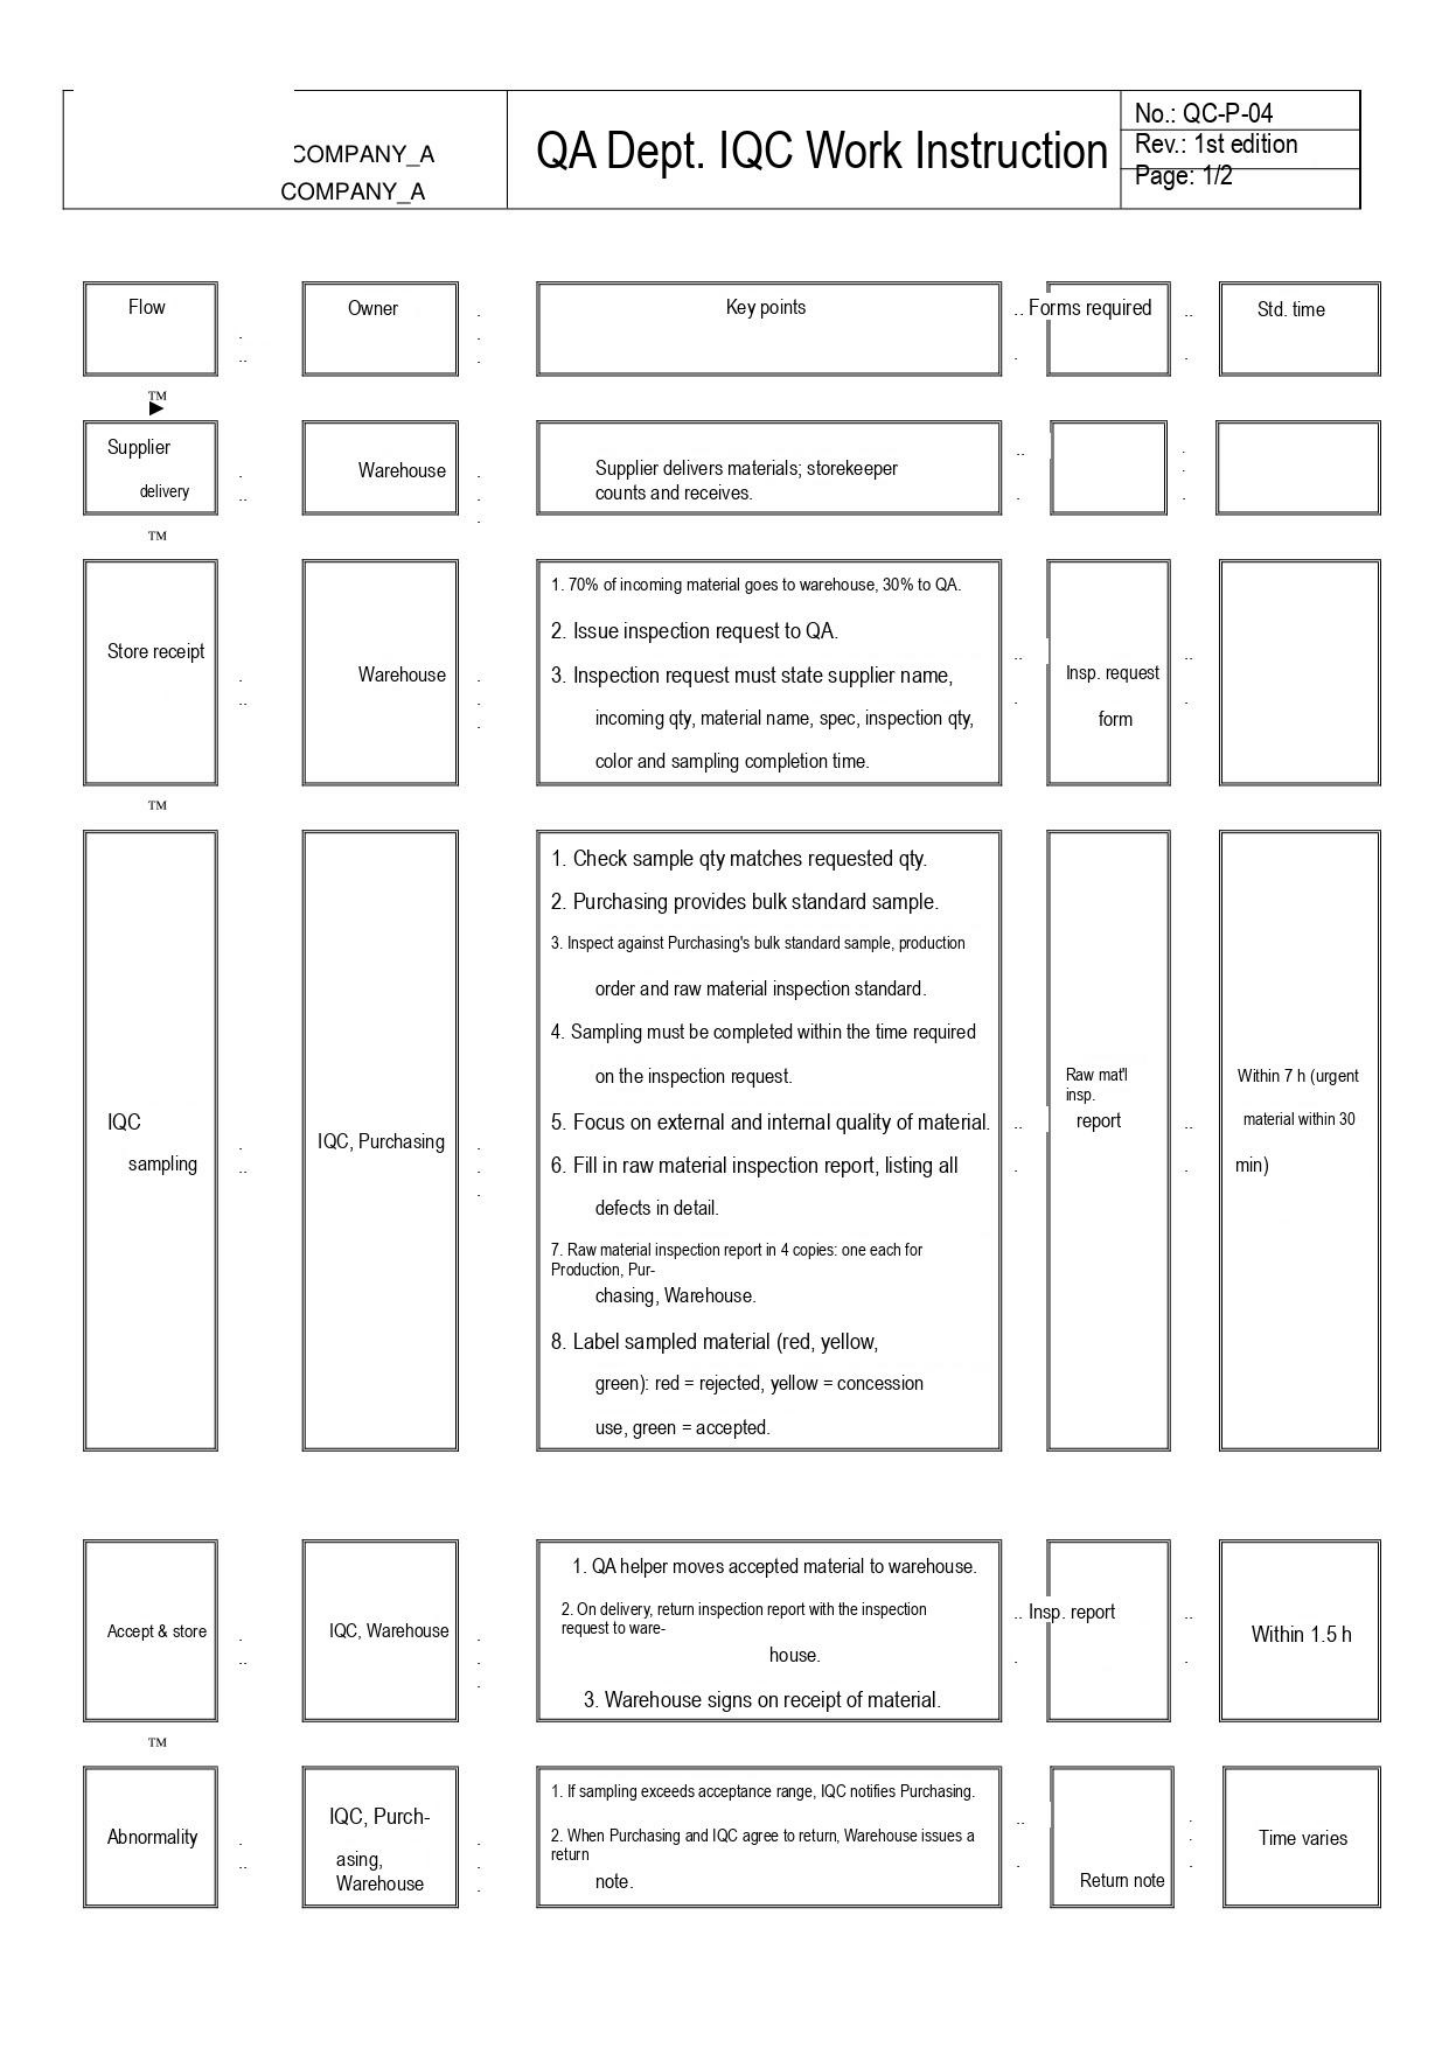COMPANY_A
COMPANY_A

QA Dept. IQC Work Instruction

No.: QC-P-04
Rev.: 1st edition
Page: 1/2

| Flow | Owner | Key points | Forms required | Std. time |
|---|---|---|---|---|
| Supplier delivery | Warehouse | Supplier delivers materials; storekeeper counts and receives. | | |
| Store receipt | Warehouse | 1. 70% of incoming material goes to warehouse, 30% to QA.<br>2. Issue inspection request to QA.<br>3. Inspection request must state supplier name, incoming qty, material name, spec, inspection qty, color and sampling completion time. | Insp. request form | |
| IQC sampling | IQC, Purchasing | 1. Check sample qty matches requested qty.<br>2. Purchasing provides bulk standard sample.<br>3. Inspect against Purchasing's bulk standard sample, production order and raw material inspection standard.<br>4. Sampling must be completed within the time required on the inspection request.<br>5. Focus on external and internal quality of material.<br>6. Fill in raw material inspection report, listing all defects in detail.<br>7. Raw material inspection report in 4 copies: one each for Production, Pur-chasing, Warehouse.<br>8. Label sampled material (red, yellow, green): red = rejected, yellow = concession use, green = accepted. | Raw mat'l insp. report | Within 7 h (urgent material within 30 min) |
| Accept & store | IQC, Warehouse | 1. QA helper moves accepted material to warehouse.<br>2. On delivery, return inspection report with the inspection request to ware-house.<br>3. Warehouse signs on receipt of material. | Insp. report | Within 1.5 h |
| Abnormality | IQC, Purch-asing, Warehouse | 1. If sampling exceeds acceptance range, IQC notifies Purchasing.<br>2. When Purchasing and IQC agree to return, Warehouse issues a return note. | Return note | Time varies |
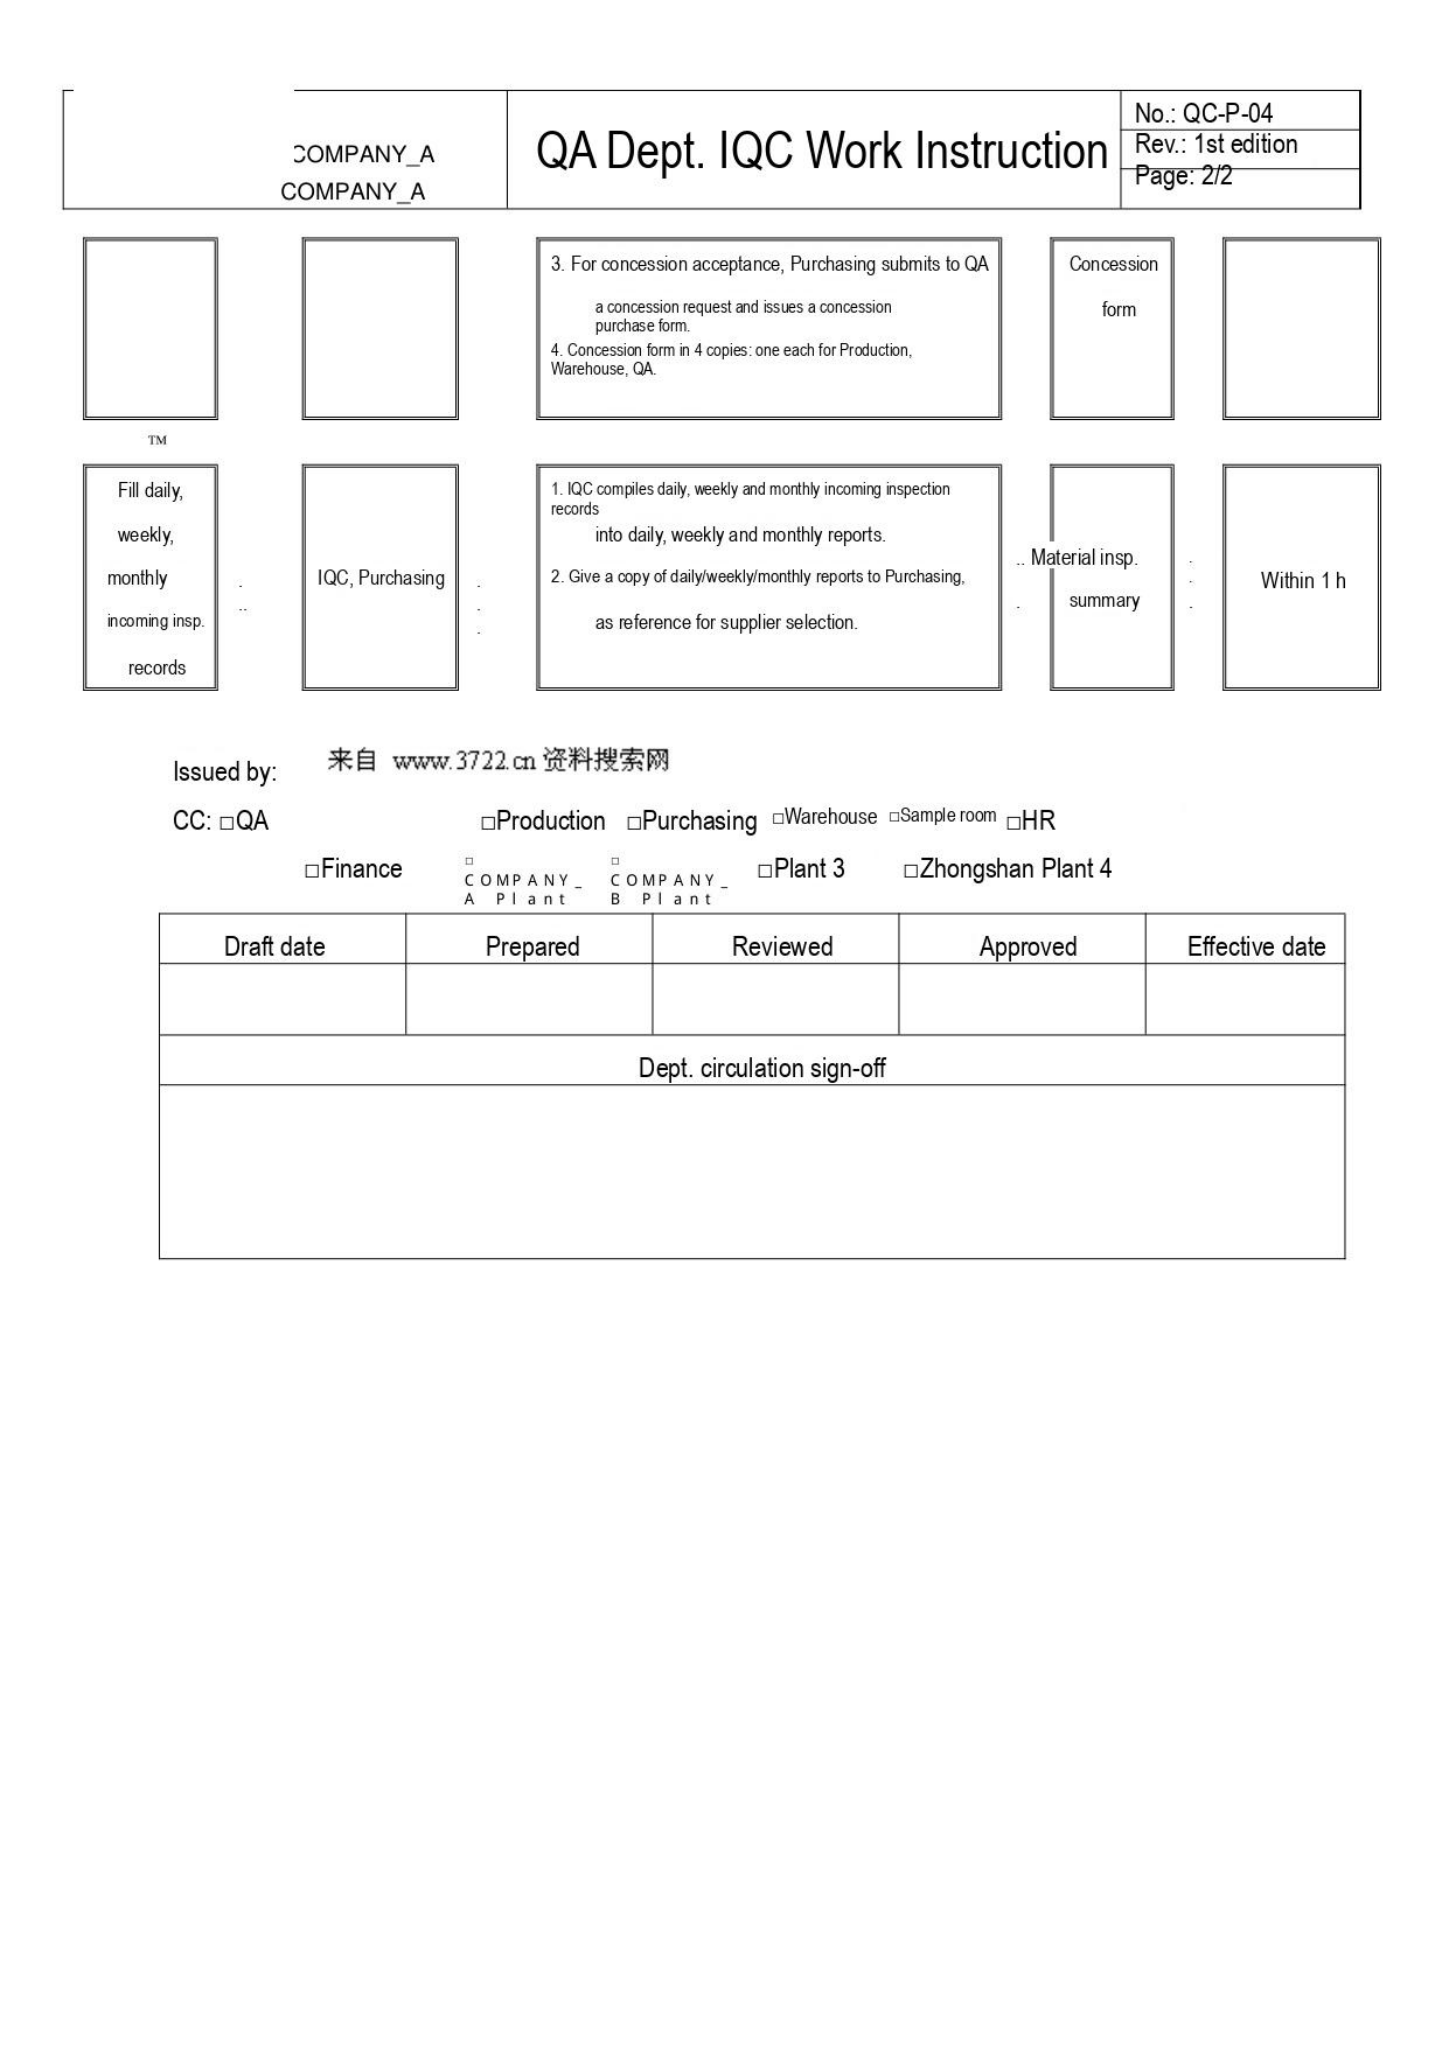COMPANY_A
COMPANY_A

QA Dept. IQC Work Instruction

No.: QC-P-04
Rev.: 1st edition
Page: 2/2

3. For concession acceptance, Purchasing submits to QA
a concession request and issues a concession purchase form.
4. Concession form in 4 copies: one each for Production, Warehouse, QA.

Concession form

TM

Fill daily, weekly, monthly incoming insp. records

IQC, Purchasing

1. IQC compiles daily, weekly and monthly incoming inspection records
into daily, weekly and monthly reports.
2. Give a copy of daily/weekly/monthly reports to Purchasing,
as reference for supplier selection.

Material insp. summary

Within 1 h

Issued by: 来自 www.3722.cn 资料搜索网

CC: □QA □Production □Purchasing □Warehouse □Sample room □HR
□Finance □COMPANY_A Plant □COMPANY_B Plant □Plant 3 □Zhongshan Plant 4

| Draft date | Prepared | Reviewed | Approved | Effective date |
|---|---|---|---|---|
| | | | | |
| Dept. circulation sign-off | | | | |
| | | | | |